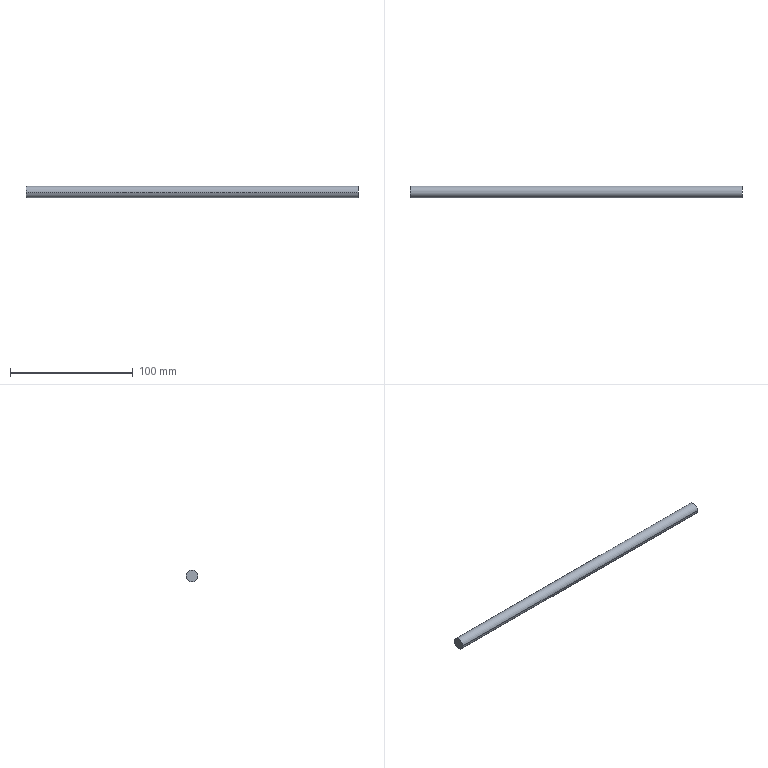Part | NX | features BREP 1 | 1 solid | 4 faces | box 271.018 x 9.525 x 9.525 mm | volume 19312 mm3 | plane 2 | cylinder 2 | commonest cylinder face diameters 9.525 x2
STEP:
#1=CARTESIAN_POINT('',(-135.509,4.763,0.));
#2=VERTEX_POINT('',#1);
#3=CARTESIAN_POINT('',(-135.509,-4.763,0.));
#4=VERTEX_POINT('',#3);
#5=CARTESIAN_POINT('',(-135.509,0.,0.));
#6=DIRECTION('',(1.,0.,0.));
#7=DIRECTION('',(0.,1.,0.));
#8=AXIS2_PLACEMENT_3D('',#5,#6,#7);
#9=CIRCLE('',#8,4.763);
#10=EDGE_CURVE('',#2,#4,#9,.T.);
#11=ORIENTED_EDGE('',*,*,#10,.F.);
#12=CARTESIAN_POINT('',(-135.509,0.,0.));
#13=DIRECTION('',(1.,0.,0.));
#14=DIRECTION('',(0.,-1.,0.));
#15=AXIS2_PLACEMENT_3D('',#12,#13,#14);
#16=CIRCLE('',#15,4.763);
#17=EDGE_CURVE('',#4,#2,#16,.T.);
#18=ORIENTED_EDGE('',*,*,#17,.F.);
#19=EDGE_LOOP('',(#11,#18));
#20=FACE_BOUND('',#19,.T.);
#21=CARTESIAN_POINT('',(-135.509,0.,0.));
#22=DIRECTION('',(1.,0.,0.));
#23=DIRECTION('',(0.,1.,0.));
#24=AXIS2_PLACEMENT_3D('',#21,#22,#23);
#25=PLANE('',#24);
#26=ADVANCED_FACE('',(#20),#25,.F.);
#27=CARTESIAN_POINT('',(135.509,4.763,0.));
#28=VERTEX_POINT('',#27);
#29=CARTESIAN_POINT('',(-135.509,4.763,0.));
#30=DIRECTION('',(1.,0.,0.));
#31=VECTOR('',#30,1000.);
#32=LINE('',#29,#31);
#33=EDGE_CURVE('',#28,#2,#32,.F.);
#34=ORIENTED_EDGE('',*,*,#33,.F.);
#35=CARTESIAN_POINT('',(135.509,-4.763,0.));
#36=VERTEX_POINT('',#35);
#37=CARTESIAN_POINT('',(135.509,0.,0.));
#38=DIRECTION('',(1.,0.,0.));
#39=DIRECTION('',(0.,-1.,0.));
#40=AXIS2_PLACEMENT_3D('',#37,#38,#39);
#41=CIRCLE('',#40,4.763);
#42=EDGE_CURVE('',#36,#28,#41,.T.);
#43=ORIENTED_EDGE('',*,*,#42,.F.);
#44=CARTESIAN_POINT('',(-135.509,-4.763,0.));
#45=DIRECTION('',(1.,0.,0.));
#46=VECTOR('',#45,1000.);
#47=LINE('',#44,#46);
#48=EDGE_CURVE('',#36,#4,#47,.F.);
#49=ORIENTED_EDGE('',*,*,#48,.T.);
#50=ORIENTED_EDGE('',*,*,#17,.T.);
#51=EDGE_LOOP('',(#34,#43,#49,#50));
#52=FACE_BOUND('',#51,.T.);
#53=CARTESIAN_POINT('',(-135.509,0.,0.));
#54=DIRECTION('',(1.,0.,0.));
#55=DIRECTION('',(0.,-1.,0.));
#56=AXIS2_PLACEMENT_3D('',#53,#54,#55);
#57=CYLINDRICAL_SURFACE('',#56,4.763);
#58=ADVANCED_FACE('',(#52),#57,.T.);
#59=ORIENTED_EDGE('',*,*,#48,.F.);
#60=CARTESIAN_POINT('',(135.509,0.,0.));
#61=DIRECTION('',(1.,0.,0.));
#62=DIRECTION('',(0.,1.,0.));
#63=AXIS2_PLACEMENT_3D('',#60,#61,#62);
#64=CIRCLE('',#63,4.763);
#65=EDGE_CURVE('',#28,#36,#64,.T.);
#66=ORIENTED_EDGE('',*,*,#65,.F.);
#67=ORIENTED_EDGE('',*,*,#33,.T.);
#68=ORIENTED_EDGE('',*,*,#10,.T.);
#69=EDGE_LOOP('',(#59,#66,#67,#68));
#70=FACE_BOUND('',#69,.T.);
#71=CARTESIAN_POINT('',(-135.509,0.,0.));
#72=DIRECTION('',(1.,0.,0.));
#73=DIRECTION('',(0.,-1.,0.));
#74=AXIS2_PLACEMENT_3D('',#71,#72,#73);
#75=CYLINDRICAL_SURFACE('',#74,4.763);
#76=ADVANCED_FACE('',(#70),#75,.T.);
#77=ORIENTED_EDGE('',*,*,#65,.T.);
#78=ORIENTED_EDGE('',*,*,#42,.T.);
#79=EDGE_LOOP('',(#77,#78));
#80=FACE_BOUND('',#79,.T.);
#81=CARTESIAN_POINT('',(135.509,0.,0.));
#82=DIRECTION('',(1.,0.,0.));
#83=DIRECTION('',(0.,1.,0.));
#84=AXIS2_PLACEMENT_3D('',#81,#82,#83);
#85=PLANE('',#84);
#86=ADVANCED_FACE('',(#80),#85,.T.);
#87=CLOSED_SHELL('',(#26,#58,#76,#86));
#88=MANIFOLD_SOLID_BREP('',#87);
#89=(LENGTH_UNIT()NAMED_UNIT(*)SI_UNIT(.MILLI.,.METRE.));
#90=UNCERTAINTY_MEASURE_WITH_UNIT(LENGTH_MEASURE(0.00001),#89,'','');
#91=(NAMED_UNIT(*)PLANE_ANGLE_UNIT()SI_UNIT($,.RADIAN.));
#92=(NAMED_UNIT(*)SI_UNIT($,.STERADIAN.)SOLID_ANGLE_UNIT());
#93=(GEOMETRIC_REPRESENTATION_CONTEXT(3)GLOBAL_UNCERTAINTY_ASSIGNED_CONTEXT((#90))GLOBAL_UNIT_ASSIGNED_CONTEXT((#89,#91,#92))REPRESENTATION_CONTEXT('',''));
#94=ADVANCED_BREP_SHAPE_REPRESENTATION('',(#88),#93);